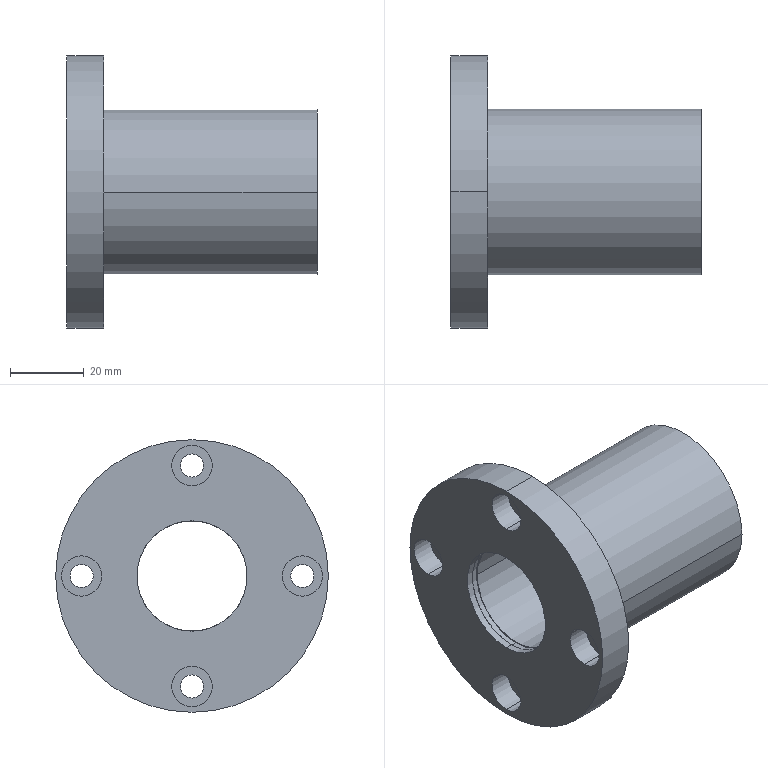Part | SolidWorks | features BaseBody 1 | 1 solid | 41 faces | box 68 x 74 x 74 mm | volume 84248 mm3 | cylinder 30 | plane 11 | commonest cylinder face diameters 6.3 x8 11 x8 30 x6 30.5 x4 45 x2 74 x2
STEP:
#1=CARTESIAN_POINT('',(0.,0.,37.));
#2=VERTEX_POINT('',#1);
#3=CARTESIAN_POINT('',(0.,0.,-37.));
#4=VERTEX_POINT('',#3);
#5=CARTESIAN_POINT('',(0.,0.,0.));
#6=DIRECTION('',(-1.,0.,0.));
#7=DIRECTION('',(0.,0.,-1.));
#8=AXIS2_PLACEMENT_3D('',#5,#6,#7);
#9=CIRCLE('',#8,37.);
#10=EDGE_CURVE('',#2,#4,#9,.T.);
#11=ORIENTED_EDGE('',*,*,#10,.F.);
#12=CARTESIAN_POINT('',(10.,0.,37.));
#13=VERTEX_POINT('',#12);
#14=CARTESIAN_POINT('',(0.,0.,37.));
#15=DIRECTION('',(1.,0.,0.));
#16=VECTOR('',#15,1000.);
#17=LINE('',#14,#16);
#18=EDGE_CURVE('',#2,#13,#17,.T.);
#19=ORIENTED_EDGE('',*,*,#18,.T.);
#20=CARTESIAN_POINT('',(10.,0.,-37.));
#21=VERTEX_POINT('',#20);
#22=CARTESIAN_POINT('',(10.,0.,0.));
#23=DIRECTION('',(1.,0.,0.));
#24=DIRECTION('',(0.,0.,-1.));
#25=AXIS2_PLACEMENT_3D('',#22,#23,#24);
#26=CIRCLE('',#25,37.);
#27=EDGE_CURVE('',#21,#13,#26,.T.);
#28=ORIENTED_EDGE('',*,*,#27,.F.);
#29=CARTESIAN_POINT('',(0.,0.,-37.));
#30=DIRECTION('',(1.,0.,0.));
#31=VECTOR('',#30,1000.);
#32=LINE('',#29,#31);
#33=EDGE_CURVE('',#4,#21,#32,.T.);
#34=ORIENTED_EDGE('',*,*,#33,.F.);
#35=EDGE_LOOP('',(#11,#19,#28,#34));
#36=FACE_OUTER_BOUND('',#35,.T.);
#37=CARTESIAN_POINT('',(0.,0.,0.));
#38=DIRECTION('',(1.,0.,0.));
#39=DIRECTION('',(0.,0.,-1.));
#40=AXIS2_PLACEMENT_3D('',#37,#38,#39);
#41=CYLINDRICAL_SURFACE('',#40,37.);
#42=ADVANCED_FACE('',(#36),#41,.T.);
#43=CARTESIAN_POINT('',(0.,0.,15.));
#44=VERTEX_POINT('',#43);
#45=CARTESIAN_POINT('',(0.,0.,-15.));
#46=VERTEX_POINT('',#45);
#47=CARTESIAN_POINT('',(0.,0.,0.));
#48=DIRECTION('',(1.,0.,0.));
#49=DIRECTION('',(0.,0.,-1.));
#50=AXIS2_PLACEMENT_3D('',#47,#48,#49);
#51=CIRCLE('',#50,15.);
#52=EDGE_CURVE('',#44,#46,#51,.T.);
#53=ORIENTED_EDGE('',*,*,#52,.F.);
#54=CARTESIAN_POINT('',(2.,0.,15.));
#55=VERTEX_POINT('',#54);
#56=CARTESIAN_POINT('',(0.,0.,15.));
#57=DIRECTION('',(1.,0.,0.));
#58=VECTOR('',#57,1000.);
#59=LINE('',#56,#58);
#60=EDGE_CURVE('',#44,#55,#59,.T.);
#61=ORIENTED_EDGE('',*,*,#60,.T.);
#62=CARTESIAN_POINT('',(2.,0.,-15.));
#63=VERTEX_POINT('',#62);
#64=CARTESIAN_POINT('',(2.,0.,0.));
#65=DIRECTION('',(1.,0.,0.));
#66=DIRECTION('',(0.,0.,-1.));
#67=AXIS2_PLACEMENT_3D('',#64,#65,#66);
#68=CIRCLE('',#67,15.);
#69=EDGE_CURVE('',#55,#63,#68,.T.);
#70=ORIENTED_EDGE('',*,*,#69,.T.);
#71=CARTESIAN_POINT('',(0.,0.,-15.));
#72=DIRECTION('',(1.,0.,0.));
#73=VECTOR('',#72,1000.);
#74=LINE('',#71,#73);
#75=EDGE_CURVE('',#46,#63,#74,.T.);
#76=ORIENTED_EDGE('',*,*,#75,.F.);
#77=EDGE_LOOP('',(#53,#61,#70,#76));
#78=FACE_OUTER_BOUND('',#77,.T.);
#79=CARTESIAN_POINT('',(0.,0.,0.));
#80=DIRECTION('',(1.,0.,0.));
#81=DIRECTION('',(0.,0.,-1.));
#82=AXIS2_PLACEMENT_3D('',#79,#80,#81);
#83=CYLINDRICAL_SURFACE('',#82,15.);
#84=ADVANCED_FACE('',(#78),#83,.F.);
#85=CARTESIAN_POINT('',(0.,30.,5.5));
#86=VERTEX_POINT('',#85);
#87=CARTESIAN_POINT('',(0.,30.,-5.5));
#88=VERTEX_POINT('',#87);
#89=CARTESIAN_POINT('',(0.,30.,0.));
#90=DIRECTION('',(1.,0.,0.));
#91=DIRECTION('',(0.,0.,-1.));
#92=AXIS2_PLACEMENT_3D('',#89,#90,#91);
#93=CIRCLE('',#92,5.5);
#94=EDGE_CURVE('',#86,#88,#93,.T.);
#95=ORIENTED_EDGE('',*,*,#94,.F.);
#96=CARTESIAN_POINT('',(6.3,30.,5.5));
#97=VERTEX_POINT('',#96);
#98=CARTESIAN_POINT('',(0.,30.,5.5));
#99=DIRECTION('',(1.,0.,0.));
#100=VECTOR('',#99,1000.);
#101=LINE('',#98,#100);
#102=EDGE_CURVE('',#86,#97,#101,.T.);
#103=ORIENTED_EDGE('',*,*,#102,.T.);
#104=CARTESIAN_POINT('',(6.3,30.,-5.5));
#105=VERTEX_POINT('',#104);
#106=CARTESIAN_POINT('',(6.3,30.,0.));
#107=DIRECTION('',(1.,0.,0.));
#108=DIRECTION('',(0.,0.,-1.));
#109=AXIS2_PLACEMENT_3D('',#106,#107,#108);
#110=CIRCLE('',#109,5.5);
#111=EDGE_CURVE('',#97,#105,#110,.T.);
#112=ORIENTED_EDGE('',*,*,#111,.T.);
#113=CARTESIAN_POINT('',(0.,30.,-5.5));
#114=DIRECTION('',(1.,0.,0.));
#115=VECTOR('',#114,1000.);
#116=LINE('',#113,#115);
#117=EDGE_CURVE('',#88,#105,#116,.T.);
#118=ORIENTED_EDGE('',*,*,#117,.F.);
#119=EDGE_LOOP('',(#95,#103,#112,#118));
#120=FACE_OUTER_BOUND('',#119,.T.);
#121=CARTESIAN_POINT('',(0.,30.,0.));
#122=DIRECTION('',(1.,0.,0.));
#123=DIRECTION('',(0.,0.,-1.));
#124=AXIS2_PLACEMENT_3D('',#121,#122,#123);
#125=CYLINDRICAL_SURFACE('',#124,5.5);
#126=ADVANCED_FACE('',(#120),#125,.F.);
#127=CARTESIAN_POINT('',(0.,0.,35.5));
#128=VERTEX_POINT('',#127);
#129=CARTESIAN_POINT('',(0.,0.,24.5));
#130=VERTEX_POINT('',#129);
#131=CARTESIAN_POINT('',(0.,0.,30.));
#132=DIRECTION('',(1.,0.,0.));
#133=DIRECTION('',(0.,0.,-1.));
#134=AXIS2_PLACEMENT_3D('',#131,#132,#133);
#135=CIRCLE('',#134,5.5);
#136=EDGE_CURVE('',#128,#130,#135,.T.);
#137=ORIENTED_EDGE('',*,*,#136,.F.);
#138=CARTESIAN_POINT('',(6.3,0.,35.5));
#139=VERTEX_POINT('',#138);
#140=CARTESIAN_POINT('',(0.,0.,35.5));
#141=DIRECTION('',(1.,0.,0.));
#142=VECTOR('',#141,1000.);
#143=LINE('',#140,#142);
#144=EDGE_CURVE('',#128,#139,#143,.T.);
#145=ORIENTED_EDGE('',*,*,#144,.T.);
#146=CARTESIAN_POINT('',(6.3,0.,24.5));
#147=VERTEX_POINT('',#146);
#148=CARTESIAN_POINT('',(6.3,0.,30.));
#149=DIRECTION('',(1.,0.,0.));
#150=DIRECTION('',(0.,0.,-1.));
#151=AXIS2_PLACEMENT_3D('',#148,#149,#150);
#152=CIRCLE('',#151,5.5);
#153=EDGE_CURVE('',#139,#147,#152,.T.);
#154=ORIENTED_EDGE('',*,*,#153,.T.);
#155=CARTESIAN_POINT('',(0.,0.,24.5));
#156=DIRECTION('',(1.,0.,0.));
#157=VECTOR('',#156,1000.);
#158=LINE('',#155,#157);
#159=EDGE_CURVE('',#130,#147,#158,.T.);
#160=ORIENTED_EDGE('',*,*,#159,.F.);
#161=EDGE_LOOP('',(#137,#145,#154,#160));
#162=FACE_OUTER_BOUND('',#161,.T.);
#163=CARTESIAN_POINT('',(0.,0.,30.));
#164=DIRECTION('',(1.,0.,0.));
#165=DIRECTION('',(0.,0.,-1.));
#166=AXIS2_PLACEMENT_3D('',#163,#164,#165);
#167=CYLINDRICAL_SURFACE('',#166,5.5);
#168=ADVANCED_FACE('',(#162),#167,.F.);
#169=CARTESIAN_POINT('',(0.,-30.,5.5));
#170=VERTEX_POINT('',#169);
#171=CARTESIAN_POINT('',(0.,-30.,-5.5));
#172=VERTEX_POINT('',#171);
#173=CARTESIAN_POINT('',(0.,-30.,0.));
#174=DIRECTION('',(1.,0.,0.));
#175=DIRECTION('',(0.,0.,-1.));
#176=AXIS2_PLACEMENT_3D('',#173,#174,#175);
#177=CIRCLE('',#176,5.5);
#178=EDGE_CURVE('',#170,#172,#177,.T.);
#179=ORIENTED_EDGE('',*,*,#178,.F.);
#180=CARTESIAN_POINT('',(6.3,-30.,5.5));
#181=VERTEX_POINT('',#180);
#182=CARTESIAN_POINT('',(0.,-30.,5.5));
#183=DIRECTION('',(1.,0.,0.));
#184=VECTOR('',#183,1000.);
#185=LINE('',#182,#184);
#186=EDGE_CURVE('',#170,#181,#185,.T.);
#187=ORIENTED_EDGE('',*,*,#186,.T.);
#188=CARTESIAN_POINT('',(6.3,-30.,-5.5));
#189=VERTEX_POINT('',#188);
#190=CARTESIAN_POINT('',(6.3,-30.,0.));
#191=DIRECTION('',(1.,0.,0.));
#192=DIRECTION('',(0.,0.,-1.));
#193=AXIS2_PLACEMENT_3D('',#190,#191,#192);
#194=CIRCLE('',#193,5.5);
#195=EDGE_CURVE('',#181,#189,#194,.T.);
#196=ORIENTED_EDGE('',*,*,#195,.T.);
#197=CARTESIAN_POINT('',(0.,-30.,-5.5));
#198=DIRECTION('',(1.,0.,0.));
#199=VECTOR('',#198,1000.);
#200=LINE('',#197,#199);
#201=EDGE_CURVE('',#172,#189,#200,.T.);
#202=ORIENTED_EDGE('',*,*,#201,.F.);
#203=EDGE_LOOP('',(#179,#187,#196,#202));
#204=FACE_OUTER_BOUND('',#203,.T.);
#205=CARTESIAN_POINT('',(0.,-30.,0.));
#206=DIRECTION('',(1.,0.,0.));
#207=DIRECTION('',(0.,0.,-1.));
#208=AXIS2_PLACEMENT_3D('',#205,#206,#207);
#209=CYLINDRICAL_SURFACE('',#208,5.5);
#210=ADVANCED_FACE('',(#204),#209,.F.);
#211=CARTESIAN_POINT('',(0.,0.,-24.5));
#212=VERTEX_POINT('',#211);
#213=CARTESIAN_POINT('',(0.,0.,-35.5));
#214=VERTEX_POINT('',#213);
#215=CARTESIAN_POINT('',(0.,0.,-30.));
#216=DIRECTION('',(1.,0.,0.));
#217=DIRECTION('',(0.,0.,-1.));
#218=AXIS2_PLACEMENT_3D('',#215,#216,#217);
#219=CIRCLE('',#218,5.5);
#220=EDGE_CURVE('',#212,#214,#219,.T.);
#221=ORIENTED_EDGE('',*,*,#220,.F.);
#222=CARTESIAN_POINT('',(6.3,0.,-24.5));
#223=VERTEX_POINT('',#222);
#224=CARTESIAN_POINT('',(0.,0.,-24.5));
#225=DIRECTION('',(1.,0.,0.));
#226=VECTOR('',#225,1000.);
#227=LINE('',#224,#226);
#228=EDGE_CURVE('',#212,#223,#227,.T.);
#229=ORIENTED_EDGE('',*,*,#228,.T.);
#230=CARTESIAN_POINT('',(6.3,0.,-35.5));
#231=VERTEX_POINT('',#230);
#232=CARTESIAN_POINT('',(6.3,0.,-30.));
#233=DIRECTION('',(1.,0.,0.));
#234=DIRECTION('',(0.,0.,-1.));
#235=AXIS2_PLACEMENT_3D('',#232,#233,#234);
#236=CIRCLE('',#235,5.5);
#237=EDGE_CURVE('',#223,#231,#236,.T.);
#238=ORIENTED_EDGE('',*,*,#237,.T.);
#239=CARTESIAN_POINT('',(0.,0.,-35.5));
#240=DIRECTION('',(1.,0.,0.));
#241=VECTOR('',#240,1000.);
#242=LINE('',#239,#241);
#243=EDGE_CURVE('',#214,#231,#242,.T.);
#244=ORIENTED_EDGE('',*,*,#243,.F.);
#245=EDGE_LOOP('',(#221,#229,#238,#244));
#246=FACE_OUTER_BOUND('',#245,.T.);
#247=CARTESIAN_POINT('',(0.,0.,-30.));
#248=DIRECTION('',(1.,0.,0.));
#249=DIRECTION('',(0.,0.,-1.));
#250=AXIS2_PLACEMENT_3D('',#247,#248,#249);
#251=CYLINDRICAL_SURFACE('',#250,5.5);
#252=ADVANCED_FACE('',(#246),#251,.F.);
#253=CARTESIAN_POINT('',(6.3,30.,-3.15));
#254=VERTEX_POINT('',#253);
#255=CARTESIAN_POINT('',(6.3,30.,3.15));
#256=VERTEX_POINT('',#255);
#257=CARTESIAN_POINT('',(6.3,30.,0.));
#258=DIRECTION('',(-1.,0.,0.));
#259=DIRECTION('',(0.,0.,-1.));
#260=AXIS2_PLACEMENT_3D('',#257,#258,#259);
#261=CIRCLE('',#260,3.15);
#262=EDGE_CURVE('',#254,#256,#261,.T.);
#263=ORIENTED_EDGE('',*,*,#262,.T.);
#264=CARTESIAN_POINT('',(10.,30.,3.15));
#265=VERTEX_POINT('',#264);
#266=CARTESIAN_POINT('',(6.3,30.,3.15));
#267=DIRECTION('',(1.,0.,0.));
#268=VECTOR('',#267,1000.);
#269=LINE('',#266,#268);
#270=EDGE_CURVE('',#256,#265,#269,.T.);
#271=ORIENTED_EDGE('',*,*,#270,.T.);
#272=CARTESIAN_POINT('',(10.,30.,-3.15));
#273=VERTEX_POINT('',#272);
#274=CARTESIAN_POINT('',(10.,30.,0.));
#275=DIRECTION('',(-1.,0.,0.));
#276=DIRECTION('',(0.,0.,-1.));
#277=AXIS2_PLACEMENT_3D('',#274,#275,#276);
#278=CIRCLE('',#277,3.15);
#279=EDGE_CURVE('',#273,#265,#278,.T.);
#280=ORIENTED_EDGE('',*,*,#279,.F.);
#281=CARTESIAN_POINT('',(6.3,30.,-3.15));
#282=DIRECTION('',(1.,0.,0.));
#283=VECTOR('',#282,1000.);
#284=LINE('',#281,#283);
#285=EDGE_CURVE('',#254,#273,#284,.T.);
#286=ORIENTED_EDGE('',*,*,#285,.F.);
#287=EDGE_LOOP('',(#263,#271,#280,#286));
#288=FACE_OUTER_BOUND('',#287,.T.);
#289=CARTESIAN_POINT('',(6.3,30.,0.));
#290=DIRECTION('',(1.,0.,0.));
#291=DIRECTION('',(0.,0.,-1.));
#292=AXIS2_PLACEMENT_3D('',#289,#290,#291);
#293=CYLINDRICAL_SURFACE('',#292,3.15);
#294=ADVANCED_FACE('',(#288),#293,.F.);
#295=CARTESIAN_POINT('',(6.3,0.,26.85));
#296=VERTEX_POINT('',#295);
#297=CARTESIAN_POINT('',(6.3,0.,33.15));
#298=VERTEX_POINT('',#297);
#299=CARTESIAN_POINT('',(6.3,0.,30.));
#300=DIRECTION('',(-1.,0.,0.));
#301=DIRECTION('',(0.,0.,-1.));
#302=AXIS2_PLACEMENT_3D('',#299,#300,#301);
#303=CIRCLE('',#302,3.15);
#304=EDGE_CURVE('',#296,#298,#303,.T.);
#305=ORIENTED_EDGE('',*,*,#304,.T.);
#306=CARTESIAN_POINT('',(10.,0.,33.15));
#307=VERTEX_POINT('',#306);
#308=CARTESIAN_POINT('',(6.3,0.,33.15));
#309=DIRECTION('',(1.,0.,0.));
#310=VECTOR('',#309,1000.);
#311=LINE('',#308,#310);
#312=EDGE_CURVE('',#298,#307,#311,.T.);
#313=ORIENTED_EDGE('',*,*,#312,.T.);
#314=CARTESIAN_POINT('',(10.,0.,26.85));
#315=VERTEX_POINT('',#314);
#316=CARTESIAN_POINT('',(10.,0.,30.));
#317=DIRECTION('',(-1.,0.,0.));
#318=DIRECTION('',(0.,0.,-1.));
#319=AXIS2_PLACEMENT_3D('',#316,#317,#318);
#320=CIRCLE('',#319,3.15);
#321=EDGE_CURVE('',#315,#307,#320,.T.);
#322=ORIENTED_EDGE('',*,*,#321,.F.);
#323=CARTESIAN_POINT('',(6.3,0.,26.85));
#324=DIRECTION('',(1.,0.,0.));
#325=VECTOR('',#324,1000.);
#326=LINE('',#323,#325);
#327=EDGE_CURVE('',#296,#315,#326,.T.);
#328=ORIENTED_EDGE('',*,*,#327,.F.);
#329=EDGE_LOOP('',(#305,#313,#322,#328));
#330=FACE_OUTER_BOUND('',#329,.T.);
#331=CARTESIAN_POINT('',(6.3,0.,30.));
#332=DIRECTION('',(1.,0.,0.));
#333=DIRECTION('',(0.,0.,-1.));
#334=AXIS2_PLACEMENT_3D('',#331,#332,#333);
#335=CYLINDRICAL_SURFACE('',#334,3.15);
#336=ADVANCED_FACE('',(#330),#335,.F.);
#337=CARTESIAN_POINT('',(6.3,-30.,-3.15));
#338=VERTEX_POINT('',#337);
#339=CARTESIAN_POINT('',(6.3,-30.,3.15));
#340=VERTEX_POINT('',#339);
#341=CARTESIAN_POINT('',(6.3,-30.,0.));
#342=DIRECTION('',(-1.,0.,0.));
#343=DIRECTION('',(0.,0.,-1.));
#344=AXIS2_PLACEMENT_3D('',#341,#342,#343);
#345=CIRCLE('',#344,3.15);
#346=EDGE_CURVE('',#338,#340,#345,.T.);
#347=ORIENTED_EDGE('',*,*,#346,.T.);
#348=CARTESIAN_POINT('',(10.,-30.,3.15));
#349=VERTEX_POINT('',#348);
#350=CARTESIAN_POINT('',(6.3,-30.,3.15));
#351=DIRECTION('',(1.,0.,0.));
#352=VECTOR('',#351,1000.);
#353=LINE('',#350,#352);
#354=EDGE_CURVE('',#340,#349,#353,.T.);
#355=ORIENTED_EDGE('',*,*,#354,.T.);
#356=CARTESIAN_POINT('',(10.,-30.,-3.15));
#357=VERTEX_POINT('',#356);
#358=CARTESIAN_POINT('',(10.,-30.,0.));
#359=DIRECTION('',(-1.,0.,0.));
#360=DIRECTION('',(0.,0.,-1.));
#361=AXIS2_PLACEMENT_3D('',#358,#359,#360);
#362=CIRCLE('',#361,3.15);
#363=EDGE_CURVE('',#357,#349,#362,.T.);
#364=ORIENTED_EDGE('',*,*,#363,.F.);
#365=CARTESIAN_POINT('',(6.3,-30.,-3.15));
#366=DIRECTION('',(1.,0.,0.));
#367=VECTOR('',#366,1000.);
#368=LINE('',#365,#367);
#369=EDGE_CURVE('',#338,#357,#368,.T.);
#370=ORIENTED_EDGE('',*,*,#369,.F.);
#371=EDGE_LOOP('',(#347,#355,#364,#370));
#372=FACE_OUTER_BOUND('',#371,.T.);
#373=CARTESIAN_POINT('',(6.3,-30.,0.));
#374=DIRECTION('',(1.,0.,0.));
#375=DIRECTION('',(0.,0.,-1.));
#376=AXIS2_PLACEMENT_3D('',#373,#374,#375);
#377=CYLINDRICAL_SURFACE('',#376,3.15);
#378=ADVANCED_FACE('',(#372),#377,.F.);
#379=CARTESIAN_POINT('',(6.3,0.,-33.15));
#380=VERTEX_POINT('',#379);
#381=CARTESIAN_POINT('',(6.3,0.,-26.85));
#382=VERTEX_POINT('',#381);
#383=CARTESIAN_POINT('',(6.3,0.,-30.));
#384=DIRECTION('',(-1.,0.,0.));
#385=DIRECTION('',(0.,0.,-1.));
#386=AXIS2_PLACEMENT_3D('',#383,#384,#385);
#387=CIRCLE('',#386,3.15);
#388=EDGE_CURVE('',#380,#382,#387,.T.);
#389=ORIENTED_EDGE('',*,*,#388,.T.);
#390=CARTESIAN_POINT('',(10.,0.,-26.85));
#391=VERTEX_POINT('',#390);
#392=CARTESIAN_POINT('',(6.3,0.,-26.85));
#393=DIRECTION('',(1.,0.,0.));
#394=VECTOR('',#393,1000.);
#395=LINE('',#392,#394);
#396=EDGE_CURVE('',#382,#391,#395,.T.);
#397=ORIENTED_EDGE('',*,*,#396,.T.);
#398=CARTESIAN_POINT('',(10.,0.,-33.15));
#399=VERTEX_POINT('',#398);
#400=CARTESIAN_POINT('',(10.,0.,-30.));
#401=DIRECTION('',(-1.,0.,0.));
#402=DIRECTION('',(0.,0.,-1.));
#403=AXIS2_PLACEMENT_3D('',#400,#401,#402);
#404=CIRCLE('',#403,3.15);
#405=EDGE_CURVE('',#399,#391,#404,.T.);
#406=ORIENTED_EDGE('',*,*,#405,.F.);
#407=CARTESIAN_POINT('',(6.3,0.,-33.15));
#408=DIRECTION('',(1.,0.,0.));
#409=VECTOR('',#408,1000.);
#410=LINE('',#407,#409);
#411=EDGE_CURVE('',#380,#399,#410,.T.);
#412=ORIENTED_EDGE('',*,*,#411,.F.);
#413=EDGE_LOOP('',(#389,#397,#406,#412));
#414=FACE_OUTER_BOUND('',#413,.T.);
#415=CARTESIAN_POINT('',(6.3,0.,-30.));
#416=DIRECTION('',(1.,0.,0.));
#417=DIRECTION('',(0.,0.,-1.));
#418=AXIS2_PLACEMENT_3D('',#415,#416,#417);
#419=CYLINDRICAL_SURFACE('',#418,3.15);
#420=ADVANCED_FACE('',(#414),#419,.F.);
#421=CARTESIAN_POINT('',(10.,-22.5,0.));
#422=VERTEX_POINT('',#421);
#423=CARTESIAN_POINT('',(10.,22.5,0.));
#424=VERTEX_POINT('',#423);
#425=CARTESIAN_POINT('',(10.,0.,0.));
#426=DIRECTION('',(-1.,0.,0.));
#427=DIRECTION('',(0.,1.,0.));
#428=AXIS2_PLACEMENT_3D('',#425,#426,#427);
#429=CIRCLE('',#428,22.5);
#430=EDGE_CURVE('',#422,#424,#429,.T.);
#431=ORIENTED_EDGE('',*,*,#430,.F.);
#432=CARTESIAN_POINT('',(68.,-22.5,0.));
#433=VERTEX_POINT('',#432);
#434=CARTESIAN_POINT('',(10.,-22.5,0.));
#435=DIRECTION('',(1.,0.,0.));
#436=VECTOR('',#435,1000.);
#437=LINE('',#434,#436);
#438=EDGE_CURVE('',#422,#433,#437,.T.);
#439=ORIENTED_EDGE('',*,*,#438,.T.);
#440=CARTESIAN_POINT('',(68.,22.5,0.));
#441=VERTEX_POINT('',#440);
#442=CARTESIAN_POINT('',(68.,0.,0.));
#443=DIRECTION('',(1.,0.,0.));
#444=DIRECTION('',(0.,1.,0.));
#445=AXIS2_PLACEMENT_3D('',#442,#443,#444);
#446=CIRCLE('',#445,22.5);
#447=EDGE_CURVE('',#441,#433,#446,.T.);
#448=ORIENTED_EDGE('',*,*,#447,.F.);
#449=CARTESIAN_POINT('',(10.,22.5,0.));
#450=DIRECTION('',(1.,0.,0.));
#451=VECTOR('',#450,1000.);
#452=LINE('',#449,#451);
#453=EDGE_CURVE('',#424,#441,#452,.T.);
#454=ORIENTED_EDGE('',*,*,#453,.F.);
#455=EDGE_LOOP('',(#431,#439,#448,#454));
#456=FACE_OUTER_BOUND('',#455,.T.);
#457=CARTESIAN_POINT('',(10.,0.,0.));
#458=DIRECTION('',(1.,0.,0.));
#459=DIRECTION('',(0.,1.,0.));
#460=AXIS2_PLACEMENT_3D('',#457,#458,#459);
#461=CYLINDRICAL_SURFACE('',#460,22.5);
#462=ADVANCED_FACE('',(#456),#461,.T.);
#463=CARTESIAN_POINT('',(2.,0.,15.25));
#464=VERTEX_POINT('',#463);
#465=CARTESIAN_POINT('',(2.,0.,-15.25));
#466=VERTEX_POINT('',#465);
#467=CARTESIAN_POINT('',(2.,0.,0.));
#468=DIRECTION('',(1.,0.,0.));
#469=DIRECTION('',(0.,0.,-1.));
#470=AXIS2_PLACEMENT_3D('',#467,#468,#469);
#471=CIRCLE('',#470,15.25);
#472=EDGE_CURVE('',#464,#466,#471,.T.);
#473=ORIENTED_EDGE('',*,*,#472,.F.);
#474=CARTESIAN_POINT('',(3.75,0.,15.25));
#475=VERTEX_POINT('',#474);
#476=CARTESIAN_POINT('',(2.,0.,15.25));
#477=DIRECTION('',(1.,0.,0.));
#478=VECTOR('',#477,1000.);
#479=LINE('',#476,#478);
#480=EDGE_CURVE('',#464,#475,#479,.T.);
#481=ORIENTED_EDGE('',*,*,#480,.T.);
#482=CARTESIAN_POINT('',(3.75,0.,-15.25));
#483=VERTEX_POINT('',#482);
#484=CARTESIAN_POINT('',(3.75,0.,0.));
#485=DIRECTION('',(1.,0.,0.));
#486=DIRECTION('',(0.,0.,-1.));
#487=AXIS2_PLACEMENT_3D('',#484,#485,#486);
#488=CIRCLE('',#487,15.25);
#489=EDGE_CURVE('',#475,#483,#488,.T.);
#490=ORIENTED_EDGE('',*,*,#489,.T.);
#491=CARTESIAN_POINT('',(2.,0.,-15.25));
#492=DIRECTION('',(1.,0.,0.));
#493=VECTOR('',#492,1000.);
#494=LINE('',#491,#493);
#495=EDGE_CURVE('',#466,#483,#494,.T.);
#496=ORIENTED_EDGE('',*,*,#495,.F.);
#497=EDGE_LOOP('',(#473,#481,#490,#496));
#498=FACE_OUTER_BOUND('',#497,.T.);
#499=CARTESIAN_POINT('',(2.,0.,0.));
#500=DIRECTION('',(1.,0.,0.));
#501=DIRECTION('',(0.,0.,-1.));
#502=AXIS2_PLACEMENT_3D('',#499,#500,#501);
#503=CYLINDRICAL_SURFACE('',#502,15.25);
#504=ADVANCED_FACE('',(#498),#503,.F.);
#505=CARTESIAN_POINT('',(66.,0.,-15.));
#506=VERTEX_POINT('',#505);
#507=CARTESIAN_POINT('',(66.,0.,15.));
#508=VERTEX_POINT('',#507);
#509=CARTESIAN_POINT('',(66.,0.,0.));
#510=DIRECTION('',(-1.,0.,0.));
#511=DIRECTION('',(0.,0.,-1.));
#512=AXIS2_PLACEMENT_3D('',#509,#510,#511);
#513=CIRCLE('',#512,15.);
#514=EDGE_CURVE('',#506,#508,#513,.T.);
#515=ORIENTED_EDGE('',*,*,#514,.T.);
#516=CARTESIAN_POINT('',(68.,0.,15.));
#517=VERTEX_POINT('',#516);
#518=CARTESIAN_POINT('',(66.,0.,15.));
#519=DIRECTION('',(1.,0.,0.));
#520=VECTOR('',#519,1000.);
#521=LINE('',#518,#520);
#522=EDGE_CURVE('',#508,#517,#521,.T.);
#523=ORIENTED_EDGE('',*,*,#522,.T.);
#524=CARTESIAN_POINT('',(68.,0.,-15.));
#525=VERTEX_POINT('',#524);
#526=CARTESIAN_POINT('',(68.,0.,0.));
#527=DIRECTION('',(-1.,0.,0.));
#528=DIRECTION('',(0.,0.,-1.));
#529=AXIS2_PLACEMENT_3D('',#526,#527,#528);
#530=CIRCLE('',#529,15.);
#531=EDGE_CURVE('',#525,#517,#530,.T.);
#532=ORIENTED_EDGE('',*,*,#531,.F.);
#533=CARTESIAN_POINT('',(66.,0.,-15.));
#534=DIRECTION('',(1.,0.,0.));
#535=VECTOR('',#534,1000.);
#536=LINE('',#533,#535);
#537=EDGE_CURVE('',#506,#525,#536,.T.);
#538=ORIENTED_EDGE('',*,*,#537,.F.);
#539=EDGE_LOOP('',(#515,#523,#532,#538));
#540=FACE_OUTER_BOUND('',#539,.T.);
#541=CARTESIAN_POINT('',(66.,0.,0.));
#542=DIRECTION('',(1.,0.,0.));
#543=DIRECTION('',(0.,0.,-1.));
#544=AXIS2_PLACEMENT_3D('',#541,#542,#543);
#545=CYLINDRICAL_SURFACE('',#544,15.);
#546=ADVANCED_FACE('',(#540),#545,.F.);
#547=CARTESIAN_POINT('',(3.75,-15.,0.));
#548=VERTEX_POINT('',#547);
#549=CARTESIAN_POINT('',(3.75,15.,0.));
#550=VERTEX_POINT('',#549);
#551=CARTESIAN_POINT('',(3.75,0.,0.));
#552=DIRECTION('',(1.,0.,0.));
#553=DIRECTION('',(0.,1.,0.));
#554=AXIS2_PLACEMENT_3D('',#551,#552,#553);
#555=CIRCLE('',#554,15.);
#556=EDGE_CURVE('',#548,#550,#555,.T.);
#557=ORIENTED_EDGE('',*,*,#556,.F.);
#558=CARTESIAN_POINT('',(64.25,-15.,0.));
#559=VERTEX_POINT('',#558);
#560=CARTESIAN_POINT('',(3.75,-15.,0.));
#561=DIRECTION('',(1.,0.,0.));
#562=VECTOR('',#561,1000.);
#563=LINE('',#560,#562);
#564=EDGE_CURVE('',#548,#559,#563,.T.);
#565=ORIENTED_EDGE('',*,*,#564,.T.);
#566=CARTESIAN_POINT('',(64.25,15.,0.));
#567=VERTEX_POINT('',#566);
#568=CARTESIAN_POINT('',(64.25,0.,0.));
#569=DIRECTION('',(1.,0.,0.));
#570=DIRECTION('',(0.,1.,0.));
#571=AXIS2_PLACEMENT_3D('',#568,#569,#570);
#572=CIRCLE('',#571,15.);
#573=EDGE_CURVE('',#559,#567,#572,.T.);
#574=ORIENTED_EDGE('',*,*,#573,.T.);
#575=CARTESIAN_POINT('',(3.75,15.,0.));
#576=DIRECTION('',(1.,0.,0.));
#577=VECTOR('',#576,1000.);
#578=LINE('',#575,#577);
#579=EDGE_CURVE('',#550,#567,#578,.T.);
#580=ORIENTED_EDGE('',*,*,#579,.F.);
#581=EDGE_LOOP('',(#557,#565,#574,#580));
#582=FACE_OUTER_BOUND('',#581,.T.);
#583=CARTESIAN_POINT('',(3.75,0.,0.));
#584=DIRECTION('',(1.,0.,0.));
#585=DIRECTION('',(0.,1.,0.));
#586=AXIS2_PLACEMENT_3D('',#583,#584,#585);
#587=CYLINDRICAL_SURFACE('',#586,15.);
#588=ADVANCED_FACE('',(#582),#587,.F.);
#589=CARTESIAN_POINT('',(64.25,0.,-15.25));
#590=VERTEX_POINT('',#589);
#591=CARTESIAN_POINT('',(64.25,0.,15.25));
#592=VERTEX_POINT('',#591);
#593=CARTESIAN_POINT('',(64.25,0.,0.));
#594=DIRECTION('',(-1.,0.,0.));
#595=DIRECTION('',(0.,0.,-1.));
#596=AXIS2_PLACEMENT_3D('',#593,#594,#595);
#597=CIRCLE('',#596,15.25);
#598=EDGE_CURVE('',#590,#592,#597,.T.);
#599=ORIENTED_EDGE('',*,*,#598,.T.);
#600=CARTESIAN_POINT('',(66.,0.,15.25));
#601=VERTEX_POINT('',#600);
#602=CARTESIAN_POINT('',(64.25,0.,15.25));
#603=DIRECTION('',(1.,0.,0.));
#604=VECTOR('',#603,1000.);
#605=LINE('',#602,#604);
#606=EDGE_CURVE('',#592,#601,#605,.T.);
#607=ORIENTED_EDGE('',*,*,#606,.T.);
#608=CARTESIAN_POINT('',(66.,0.,-15.25));
#609=VERTEX_POINT('',#608);
#610=CARTESIAN_POINT('',(66.,0.,0.));
#611=DIRECTION('',(-1.,0.,0.));
#612=DIRECTION('',(0.,0.,-1.));
#613=AXIS2_PLACEMENT_3D('',#610,#611,#612);
#614=CIRCLE('',#613,15.25);
#615=EDGE_CURVE('',#609,#601,#614,.T.);
#616=ORIENTED_EDGE('',*,*,#615,.F.);
#617=CARTESIAN_POINT('',(64.25,0.,-15.25));
#618=DIRECTION('',(1.,0.,0.));
#619=VECTOR('',#618,1000.);
#620=LINE('',#617,#619);
#621=EDGE_CURVE('',#590,#609,#620,.T.);
#622=ORIENTED_EDGE('',*,*,#621,.F.);
#623=EDGE_LOOP('',(#599,#607,#616,#622));
#624=FACE_OUTER_BOUND('',#623,.T.);
#625=CARTESIAN_POINT('',(64.25,0.,0.));
#626=DIRECTION('',(1.,0.,0.));
#627=DIRECTION('',(0.,0.,-1.));
#628=AXIS2_PLACEMENT_3D('',#625,#626,#627);
#629=CYLINDRICAL_SURFACE('',#628,15.25);
#630=ADVANCED_FACE('',(#624),#629,.F.);
#631=ORIENTED_EDGE('',*,*,#18,.F.);
#632=CARTESIAN_POINT('',(0.,0.,0.));
#633=DIRECTION('',(-1.,0.,0.));
#634=DIRECTION('',(0.,0.,-1.));
#635=AXIS2_PLACEMENT_3D('',#632,#633,#634);
#636=CIRCLE('',#635,37.);
#637=EDGE_CURVE('',#4,#2,#636,.T.);
#638=ORIENTED_EDGE('',*,*,#637,.F.);
#639=ORIENTED_EDGE('',*,*,#33,.T.);
#640=CARTESIAN_POINT('',(10.,0.,0.));
#641=DIRECTION('',(1.,0.,0.));
#642=DIRECTION('',(0.,0.,-1.));
#643=AXIS2_PLACEMENT_3D('',#640,#641,#642);
#644=CIRCLE('',#643,37.);
#645=EDGE_CURVE('',#13,#21,#644,.T.);
#646=ORIENTED_EDGE('',*,*,#645,.F.);
#647=EDGE_LOOP('',(#631,#638,#639,#646));
#648=FACE_OUTER_BOUND('',#647,.T.);
#649=CARTESIAN_POINT('',(0.,0.,0.));
#650=DIRECTION('',(1.,0.,0.));
#651=DIRECTION('',(0.,0.,-1.));
#652=AXIS2_PLACEMENT_3D('',#649,#650,#651);
#653=CYLINDRICAL_SURFACE('',#652,37.);
#654=ADVANCED_FACE('',(#648),#653,.T.);
#655=CARTESIAN_POINT('',(0.,0.,0.));
#656=DIRECTION('',(1.,0.,0.));
#657=DIRECTION('',(0.,0.,-1.));
#658=AXIS2_PLACEMENT_3D('',#655,#656,#657);
#659=CIRCLE('',#658,15.);
#660=EDGE_CURVE('',#46,#44,#659,.T.);
#661=ORIENTED_EDGE('',*,*,#660,.T.);
#662=ORIENTED_EDGE('',*,*,#52,.T.);
#663=EDGE_LOOP('',(#661,#662));
#664=FACE_BOUND('',#663,.T.);
#665=CARTESIAN_POINT('',(0.,30.,0.));
#666=DIRECTION('',(1.,0.,0.));
#667=DIRECTION('',(0.,0.,-1.));
#668=AXIS2_PLACEMENT_3D('',#665,#666,#667);
#669=CIRCLE('',#668,5.5);
#670=EDGE_CURVE('',#88,#86,#669,.T.);
#671=ORIENTED_EDGE('',*,*,#670,.T.);
#672=ORIENTED_EDGE('',*,*,#94,.T.);
#673=EDGE_LOOP('',(#671,#672));
#674=FACE_BOUND('',#673,.T.);
#675=CARTESIAN_POINT('',(0.,0.,30.));
#676=DIRECTION('',(1.,0.,0.));
#677=DIRECTION('',(0.,0.,-1.));
#678=AXIS2_PLACEMENT_3D('',#675,#676,#677);
#679=CIRCLE('',#678,5.5);
#680=EDGE_CURVE('',#130,#128,#679,.T.);
#681=ORIENTED_EDGE('',*,*,#680,.T.);
#682=ORIENTED_EDGE('',*,*,#136,.T.);
#683=EDGE_LOOP('',(#681,#682));
#684=FACE_BOUND('',#683,.T.);
#685=CARTESIAN_POINT('',(0.,-30.,0.));
#686=DIRECTION('',(1.,0.,0.));
#687=DIRECTION('',(0.,0.,-1.));
#688=AXIS2_PLACEMENT_3D('',#685,#686,#687);
#689=CIRCLE('',#688,5.5);
#690=EDGE_CURVE('',#172,#170,#689,.T.);
#691=ORIENTED_EDGE('',*,*,#690,.T.);
#692=ORIENTED_EDGE('',*,*,#178,.T.);
#693=EDGE_LOOP('',(#691,#692));
#694=FACE_BOUND('',#693,.T.);
#695=CARTESIAN_POINT('',(0.,0.,-30.));
#696=DIRECTION('',(1.,0.,0.));
#697=DIRECTION('',(0.,0.,-1.));
#698=AXIS2_PLACEMENT_3D('',#695,#696,#697);
#699=CIRCLE('',#698,5.5);
#700=EDGE_CURVE('',#214,#212,#699,.T.);
#701=ORIENTED_EDGE('',*,*,#700,.T.);
#702=ORIENTED_EDGE('',*,*,#220,.T.);
#703=EDGE_LOOP('',(#701,#702));
#704=FACE_BOUND('',#703,.T.);
#705=ORIENTED_EDGE('',*,*,#637,.T.);
#706=ORIENTED_EDGE('',*,*,#10,.T.);
#707=EDGE_LOOP('',(#705,#706));
#708=FACE_OUTER_BOUND('',#707,.T.);
#709=CARTESIAN_POINT('',(0.,-37.444,-37.444));
#710=DIRECTION('',(-1.,0.,0.));
#711=DIRECTION('',(0.,0.,1.));
#712=AXIS2_PLACEMENT_3D('',#709,#710,#711);
#713=PLANE('',#712);
#714=ADVANCED_FACE('',(#664,#674,#684,#694,#704,#708),#713,.T.);
#715=ORIENTED_EDGE('',*,*,#279,.T.);
#716=CARTESIAN_POINT('',(10.,30.,0.));
#717=DIRECTION('',(-1.,0.,0.));
#718=DIRECTION('',(0.,0.,-1.));
#719=AXIS2_PLACEMENT_3D('',#716,#717,#718);
#720=CIRCLE('',#719,3.15);
#721=EDGE_CURVE('',#265,#273,#720,.T.);
#722=ORIENTED_EDGE('',*,*,#721,.T.);
#723=EDGE_LOOP('',(#715,#722));
#724=FACE_BOUND('',#723,.T.);
#725=ORIENTED_EDGE('',*,*,#321,.T.);
#726=CARTESIAN_POINT('',(10.,0.,30.));
#727=DIRECTION('',(-1.,0.,0.));
#728=DIRECTION('',(0.,0.,-1.));
#729=AXIS2_PLACEMENT_3D('',#726,#727,#728);
#730=CIRCLE('',#729,3.15);
#731=EDGE_CURVE('',#307,#315,#730,.T.);
#732=ORIENTED_EDGE('',*,*,#731,.T.);
#733=EDGE_LOOP('',(#725,#732));
#734=FACE_BOUND('',#733,.T.);
#735=ORIENTED_EDGE('',*,*,#363,.T.);
#736=CARTESIAN_POINT('',(10.,-30.,0.));
#737=DIRECTION('',(-1.,0.,0.));
#738=DIRECTION('',(0.,0.,-1.));
#739=AXIS2_PLACEMENT_3D('',#736,#737,#738);
#740=CIRCLE('',#739,3.15);
#741=EDGE_CURVE('',#349,#357,#740,.T.);
#742=ORIENTED_EDGE('',*,*,#741,.T.);
#743=EDGE_LOOP('',(#735,#742));
#744=FACE_BOUND('',#743,.T.);
#745=ORIENTED_EDGE('',*,*,#405,.T.);
#746=CARTESIAN_POINT('',(10.,0.,-30.));
#747=DIRECTION('',(-1.,0.,0.));
#748=DIRECTION('',(0.,0.,-1.));
#749=AXIS2_PLACEMENT_3D('',#746,#747,#748);
#750=CIRCLE('',#749,3.15);
#751=EDGE_CURVE('',#391,#399,#750,.T.);
#752=ORIENTED_EDGE('',*,*,#751,.T.);
#753=EDGE_LOOP('',(#745,#752));
#754=FACE_BOUND('',#753,.T.);
#755=CARTESIAN_POINT('',(10.,0.,0.));
#756=DIRECTION('',(-1.,0.,0.));
#757=DIRECTION('',(0.,1.,0.));
#758=AXIS2_PLACEMENT_3D('',#755,#756,#757);
#759=CIRCLE('',#758,22.5);
#760=EDGE_CURVE('',#424,#422,#759,.T.);
#761=ORIENTED_EDGE('',*,*,#760,.T.);
#762=ORIENTED_EDGE('',*,*,#430,.T.);
#763=EDGE_LOOP('',(#761,#762));
#764=FACE_BOUND('',#763,.T.);
#765=ORIENTED_EDGE('',*,*,#27,.T.);
#766=ORIENTED_EDGE('',*,*,#645,.T.);
#767=EDGE_LOOP('',(#765,#766));
#768=FACE_OUTER_BOUND('',#767,.T.);
#769=CARTESIAN_POINT('',(10.,-37.444,-37.444));
#770=DIRECTION('',(1.,0.,0.));
#771=DIRECTION('',(0.,1.,0.));
#772=AXIS2_PLACEMENT_3D('',#769,#770,#771);
#773=PLANE('',#772);
#774=ADVANCED_FACE('',(#724,#734,#744,#754,#764,#768),#773,.T.);
#775=ORIENTED_EDGE('',*,*,#60,.F.);
#776=ORIENTED_EDGE('',*,*,#660,.F.);
#777=ORIENTED_EDGE('',*,*,#75,.T.);
#778=CARTESIAN_POINT('',(2.,0.,0.));
#779=DIRECTION('',(1.,0.,0.));
#780=DIRECTION('',(0.,0.,-1.));
#781=AXIS2_PLACEMENT_3D('',#778,#779,#780);
#782=CIRCLE('',#781,15.);
#783=EDGE_CURVE('',#63,#55,#782,.T.);
#784=ORIENTED_EDGE('',*,*,#783,.T.);
#785=EDGE_LOOP('',(#775,#776,#777,#784));
#786=FACE_OUTER_BOUND('',#785,.T.);
#787=CARTESIAN_POINT('',(0.,0.,0.));
#788=DIRECTION('',(1.,0.,0.));
#789=DIRECTION('',(0.,0.,-1.));
#790=AXIS2_PLACEMENT_3D('',#787,#788,#789);
#791=CYLINDRICAL_SURFACE('',#790,15.);
#792=ADVANCED_FACE('',(#786),#791,.F.);
#793=ORIENTED_EDGE('',*,*,#102,.F.);
#794=ORIENTED_EDGE('',*,*,#670,.F.);
#795=ORIENTED_EDGE('',*,*,#117,.T.);
#796=CARTESIAN_POINT('',(6.3,30.,0.));
#797=DIRECTION('',(1.,0.,0.));
#798=DIRECTION('',(0.,0.,-1.));
#799=AXIS2_PLACEMENT_3D('',#796,#797,#798);
#800=CIRCLE('',#799,5.5);
#801=EDGE_CURVE('',#105,#97,#800,.T.);
#802=ORIENTED_EDGE('',*,*,#801,.T.);
#803=EDGE_LOOP('',(#793,#794,#795,#802));
#804=FACE_OUTER_BOUND('',#803,.T.);
#805=CARTESIAN_POINT('',(0.,30.,0.));
#806=DIRECTION('',(1.,0.,0.));
#807=DIRECTION('',(0.,0.,-1.));
#808=AXIS2_PLACEMENT_3D('',#805,#806,#807);
#809=CYLINDRICAL_SURFACE('',#808,5.5);
#810=ADVANCED_FACE('',(#804),#809,.F.);
#811=ORIENTED_EDGE('',*,*,#144,.F.);
#812=ORIENTED_EDGE('',*,*,#680,.F.);
#813=ORIENTED_EDGE('',*,*,#159,.T.);
#814=CARTESIAN_POINT('',(6.3,0.,30.));
#815=DIRECTION('',(1.,0.,0.));
#816=DIRECTION('',(0.,0.,-1.));
#817=AXIS2_PLACEMENT_3D('',#814,#815,#816);
#818=CIRCLE('',#817,5.5);
#819=EDGE_CURVE('',#147,#139,#818,.T.);
#820=ORIENTED_EDGE('',*,*,#819,.T.);
#821=EDGE_LOOP('',(#811,#812,#813,#820));
#822=FACE_OUTER_BOUND('',#821,.T.);
#823=CARTESIAN_POINT('',(0.,0.,30.));
#824=DIRECTION('',(1.,0.,0.));
#825=DIRECTION('',(0.,0.,-1.));
#826=AXIS2_PLACEMENT_3D('',#823,#824,#825);
#827=CYLINDRICAL_SURFACE('',#826,5.5);
#828=ADVANCED_FACE('',(#822),#827,.F.);
#829=ORIENTED_EDGE('',*,*,#186,.F.);
#830=ORIENTED_EDGE('',*,*,#690,.F.);
#831=ORIENTED_EDGE('',*,*,#201,.T.);
#832=CARTESIAN_POINT('',(6.3,-30.,0.));
#833=DIRECTION('',(1.,0.,0.));
#834=DIRECTION('',(0.,0.,-1.));
#835=AXIS2_PLACEMENT_3D('',#832,#833,#834);
#836=CIRCLE('',#835,5.5);
#837=EDGE_CURVE('',#189,#181,#836,.T.);
#838=ORIENTED_EDGE('',*,*,#837,.T.);
#839=EDGE_LOOP('',(#829,#830,#831,#838));
#840=FACE_OUTER_BOUND('',#839,.T.);
#841=CARTESIAN_POINT('',(0.,-30.,0.));
#842=DIRECTION('',(1.,0.,0.));
#843=DIRECTION('',(0.,0.,-1.));
#844=AXIS2_PLACEMENT_3D('',#841,#842,#843);
#845=CYLINDRICAL_SURFACE('',#844,5.5);
#846=ADVANCED_FACE('',(#840),#845,.F.);
#847=ORIENTED_EDGE('',*,*,#228,.F.);
#848=ORIENTED_EDGE('',*,*,#700,.F.);
#849=ORIENTED_EDGE('',*,*,#243,.T.);
#850=CARTESIAN_POINT('',(6.3,0.,-30.));
#851=DIRECTION('',(1.,0.,0.));
#852=DIRECTION('',(0.,0.,-1.));
#853=AXIS2_PLACEMENT_3D('',#850,#851,#852);
#854=CIRCLE('',#853,5.5);
#855=EDGE_CURVE('',#231,#223,#854,.T.);
#856=ORIENTED_EDGE('',*,*,#855,.T.);
#857=EDGE_LOOP('',(#847,#848,#849,#856));
#858=FACE_OUTER_BOUND('',#857,.T.);
#859=CARTESIAN_POINT('',(0.,0.,-30.));
#860=DIRECTION('',(1.,0.,0.));
#861=DIRECTION('',(0.,0.,-1.));
#862=AXIS2_PLACEMENT_3D('',#859,#860,#861);
#863=CYLINDRICAL_SURFACE('',#862,5.5);
#864=ADVANCED_FACE('',(#858),#863,.F.);
#865=ORIENTED_EDGE('',*,*,#270,.F.);
#866=CARTESIAN_POINT('',(6.3,30.,0.));
#867=DIRECTION('',(-1.,0.,0.));
#868=DIRECTION('',(0.,0.,-1.));
#869=AXIS2_PLACEMENT_3D('',#866,#867,#868);
#870=CIRCLE('',#869,3.15);
#871=EDGE_CURVE('',#256,#254,#870,.T.);
#872=ORIENTED_EDGE('',*,*,#871,.T.);
#873=ORIENTED_EDGE('',*,*,#285,.T.);
#874=ORIENTED_EDGE('',*,*,#721,.F.);
#875=EDGE_LOOP('',(#865,#872,#873,#874));
#876=FACE_OUTER_BOUND('',#875,.T.);
#877=CARTESIAN_POINT('',(6.3,30.,0.));
#878=DIRECTION('',(1.,0.,0.));
#879=DIRECTION('',(0.,0.,-1.));
#880=AXIS2_PLACEMENT_3D('',#877,#878,#879);
#881=CYLINDRICAL_SURFACE('',#880,3.15);
#882=ADVANCED_FACE('',(#876),#881,.F.);
#883=ORIENTED_EDGE('',*,*,#312,.F.);
#884=CARTESIAN_POINT('',(6.3,0.,30.));
#885=DIRECTION('',(-1.,0.,0.));
#886=DIRECTION('',(0.,0.,-1.));
#887=AXIS2_PLACEMENT_3D('',#884,#885,#886);
#888=CIRCLE('',#887,3.15);
#889=EDGE_CURVE('',#298,#296,#888,.T.);
#890=ORIENTED_EDGE('',*,*,#889,.T.);
#891=ORIENTED_EDGE('',*,*,#327,.T.);
#892=ORIENTED_EDGE('',*,*,#731,.F.);
#893=EDGE_LOOP('',(#883,#890,#891,#892));
#894=FACE_OUTER_BOUND('',#893,.T.);
#895=CARTESIAN_POINT('',(6.3,0.,30.));
#896=DIRECTION('',(1.,0.,0.));
#897=DIRECTION('',(0.,0.,-1.));
#898=AXIS2_PLACEMENT_3D('',#895,#896,#897);
#899=CYLINDRICAL_SURFACE('',#898,3.15);
#900=ADVANCED_FACE('',(#894),#899,.F.);
#901=ORIENTED_EDGE('',*,*,#354,.F.);
#902=CARTESIAN_POINT('',(6.3,-30.,0.));
#903=DIRECTION('',(-1.,0.,0.));
#904=DIRECTION('',(0.,0.,-1.));
#905=AXIS2_PLACEMENT_3D('',#902,#903,#904);
#906=CIRCLE('',#905,3.15);
#907=EDGE_CURVE('',#340,#338,#906,.T.);
#908=ORIENTED_EDGE('',*,*,#907,.T.);
#909=ORIENTED_EDGE('',*,*,#369,.T.);
#910=ORIENTED_EDGE('',*,*,#741,.F.);
#911=EDGE_LOOP('',(#901,#908,#909,#910));
#912=FACE_OUTER_BOUND('',#911,.T.);
#913=CARTESIAN_POINT('',(6.3,-30.,0.));
#914=DIRECTION('',(1.,0.,0.));
#915=DIRECTION('',(0.,0.,-1.));
#916=AXIS2_PLACEMENT_3D('',#913,#914,#915);
#917=CYLINDRICAL_SURFACE('',#916,3.15);
#918=ADVANCED_FACE('',(#912),#917,.F.);
#919=ORIENTED_EDGE('',*,*,#396,.F.);
#920=CARTESIAN_POINT('',(6.3,0.,-30.));
#921=DIRECTION('',(-1.,0.,0.));
#922=DIRECTION('',(0.,0.,-1.));
#923=AXIS2_PLACEMENT_3D('',#920,#921,#922);
#924=CIRCLE('',#923,3.15);
#925=EDGE_CURVE('',#382,#380,#924,.T.);
#926=ORIENTED_EDGE('',*,*,#925,.T.);
#927=ORIENTED_EDGE('',*,*,#411,.T.);
#928=ORIENTED_EDGE('',*,*,#751,.F.);
#929=EDGE_LOOP('',(#919,#926,#927,#928));
#930=FACE_OUTER_BOUND('',#929,.T.);
#931=CARTESIAN_POINT('',(6.3,0.,-30.));
#932=DIRECTION('',(1.,0.,0.));
#933=DIRECTION('',(0.,0.,-1.));
#934=AXIS2_PLACEMENT_3D('',#931,#932,#933);
#935=CYLINDRICAL_SURFACE('',#934,3.15);
#936=ADVANCED_FACE('',(#930),#935,.F.);
#937=ORIENTED_EDGE('',*,*,#438,.F.);
#938=ORIENTED_EDGE('',*,*,#760,.F.);
#939=ORIENTED_EDGE('',*,*,#453,.T.);
#940=CARTESIAN_POINT('',(68.,0.,0.));
#941=DIRECTION('',(1.,0.,0.));
#942=DIRECTION('',(0.,1.,0.));
#943=AXIS2_PLACEMENT_3D('',#940,#941,#942);
#944=CIRCLE('',#943,22.5);
#945=EDGE_CURVE('',#433,#441,#944,.T.);
#946=ORIENTED_EDGE('',*,*,#945,.F.);
#947=EDGE_LOOP('',(#937,#938,#939,#946));
#948=FACE_OUTER_BOUND('',#947,.T.);
#949=CARTESIAN_POINT('',(10.,0.,0.));
#950=DIRECTION('',(1.,0.,0.));
#951=DIRECTION('',(0.,1.,0.));
#952=AXIS2_PLACEMENT_3D('',#949,#950,#951);
#953=CYLINDRICAL_SURFACE('',#952,22.5);
#954=ADVANCED_FACE('',(#948),#953,.T.);
#955=ORIENTED_EDGE('',*,*,#783,.F.);
#956=ORIENTED_EDGE('',*,*,#69,.F.);
#957=EDGE_LOOP('',(#955,#956));
#958=FACE_BOUND('',#957,.T.);
#959=CARTESIAN_POINT('',(2.,0.,0.));
#960=DIRECTION('',(1.,0.,0.));
#961=DIRECTION('',(0.,0.,-1.));
#962=AXIS2_PLACEMENT_3D('',#959,#960,#961);
#963=CIRCLE('',#962,15.25);
#964=EDGE_CURVE('',#466,#464,#963,.T.);
#965=ORIENTED_EDGE('',*,*,#964,.T.);
#966=ORIENTED_EDGE('',*,*,#472,.T.);
#967=EDGE_LOOP('',(#965,#966));
#968=FACE_OUTER_BOUND('',#967,.T.);
#969=CARTESIAN_POINT('',(2.,-15.433,-15.433));
#970=DIRECTION('',(1.,0.,0.));
#971=DIRECTION('',(0.,1.,0.));
#972=AXIS2_PLACEMENT_3D('',#969,#970,#971);
#973=PLANE('',#972);
#974=ADVANCED_FACE('',(#958,#968),#973,.T.);
#975=ORIENTED_EDGE('',*,*,#262,.F.);
#976=ORIENTED_EDGE('',*,*,#871,.F.);
#977=EDGE_LOOP('',(#975,#976));
#978=FACE_BOUND('',#977,.T.);
#979=ORIENTED_EDGE('',*,*,#801,.F.);
#980=ORIENTED_EDGE('',*,*,#111,.F.);
#981=EDGE_LOOP('',(#979,#980));
#982=FACE_OUTER_BOUND('',#981,.T.);
#983=CARTESIAN_POINT('',(6.3,24.434,-5.566));
#984=DIRECTION('',(-1.,0.,0.));
#985=DIRECTION('',(0.,0.,1.));
#986=AXIS2_PLACEMENT_3D('',#983,#984,#985);
#987=PLANE('',#986);
#988=ADVANCED_FACE('',(#978,#982),#987,.T.);
#989=ORIENTED_EDGE('',*,*,#304,.F.);
#990=ORIENTED_EDGE('',*,*,#889,.F.);
#991=EDGE_LOOP('',(#989,#990));
#992=FACE_BOUND('',#991,.T.);
#993=ORIENTED_EDGE('',*,*,#819,.F.);
#994=ORIENTED_EDGE('',*,*,#153,.F.);
#995=EDGE_LOOP('',(#993,#994));
#996=FACE_OUTER_BOUND('',#995,.T.);
#997=CARTESIAN_POINT('',(6.3,-5.566,24.434));
#998=DIRECTION('',(-1.,0.,0.));
#999=DIRECTION('',(0.,0.,1.));
#1000=AXIS2_PLACEMENT_3D('',#997,#998,#999);
#1001=PLANE('',#1000);
#1002=ADVANCED_FACE('',(#992,#996),#1001,.T.);
#1003=ORIENTED_EDGE('',*,*,#346,.F.);
#1004=ORIENTED_EDGE('',*,*,#907,.F.);
#1005=EDGE_LOOP('',(#1003,#1004));
#1006=FACE_BOUND('',#1005,.T.);
#1007=ORIENTED_EDGE('',*,*,#837,.F.);
#1008=ORIENTED_EDGE('',*,*,#195,.F.);
#1009=EDGE_LOOP('',(#1007,#1008));
#1010=FACE_OUTER_BOUND('',#1009,.T.);
#1011=CARTESIAN_POINT('',(6.3,-35.566,-5.566));
#1012=DIRECTION('',(-1.,0.,0.));
#1013=DIRECTION('',(0.,0.,1.));
#1014=AXIS2_PLACEMENT_3D('',#1011,#1012,#1013);
#1015=PLANE('',#1014);
#1016=ADVANCED_FACE('',(#1006,#1010),#1015,.T.);
#1017=ORIENTED_EDGE('',*,*,#388,.F.);
#1018=ORIENTED_EDGE('',*,*,#925,.F.);
#1019=EDGE_LOOP('',(#1017,#1018));
#1020=FACE_BOUND('',#1019,.T.);
#1021=ORIENTED_EDGE('',*,*,#855,.F.);
#1022=ORIENTED_EDGE('',*,*,#237,.F.);
#1023=EDGE_LOOP('',(#1021,#1022));
#1024=FACE_OUTER_BOUND('',#1023,.T.);
#1025=CARTESIAN_POINT('',(6.3,-5.566,-35.566));
#1026=DIRECTION('',(-1.,0.,0.));
#1027=DIRECTION('',(0.,0.,1.));
#1028=AXIS2_PLACEMENT_3D('',#1025,#1026,#1027);
#1029=PLANE('',#1028);
#1030=ADVANCED_FACE('',(#1020,#1024),#1029,.T.);
#1031=ORIENTED_EDGE('',*,*,#531,.T.);
#1032=CARTESIAN_POINT('',(68.,0.,0.));
#1033=DIRECTION('',(-1.,0.,0.));
#1034=DIRECTION('',(0.,0.,-1.));
#1035=AXIS2_PLACEMENT_3D('',#1032,#1033,#1034);
#1036=CIRCLE('',#1035,15.);
#1037=EDGE_CURVE('',#517,#525,#1036,.T.);
#1038=ORIENTED_EDGE('',*,*,#1037,.T.);
#1039=EDGE_LOOP('',(#1031,#1038));
#1040=FACE_BOUND('',#1039,.T.);
#1041=ORIENTED_EDGE('',*,*,#447,.T.);
#1042=ORIENTED_EDGE('',*,*,#945,.T.);
#1043=EDGE_LOOP('',(#1041,#1042));
#1044=FACE_OUTER_BOUND('',#1043,.T.);
#1045=CARTESIAN_POINT('',(68.,-22.77,-22.77));
#1046=DIRECTION('',(1.,0.,0.));
#1047=DIRECTION('',(0.,1.,0.));
#1048=AXIS2_PLACEMENT_3D('',#1045,#1046,#1047);
#1049=PLANE('',#1048);
#1050=ADVANCED_FACE('',(#1040,#1044),#1049,.T.);
#1051=ORIENTED_EDGE('',*,*,#480,.F.);
#1052=ORIENTED_EDGE('',*,*,#964,.F.);
#1053=ORIENTED_EDGE('',*,*,#495,.T.);
#1054=CARTESIAN_POINT('',(3.75,0.,0.));
#1055=DIRECTION('',(1.,0.,0.));
#1056=DIRECTION('',(0.,0.,-1.));
#1057=AXIS2_PLACEMENT_3D('',#1054,#1055,#1056);
#1058=CIRCLE('',#1057,15.25);
#1059=EDGE_CURVE('',#483,#475,#1058,.T.);
#1060=ORIENTED_EDGE('',*,*,#1059,.T.);
#1061=EDGE_LOOP('',(#1051,#1052,#1053,#1060));
#1062=FACE_OUTER_BOUND('',#1061,.T.);
#1063=CARTESIAN_POINT('',(2.,0.,0.));
#1064=DIRECTION('',(1.,0.,0.));
#1065=DIRECTION('',(0.,0.,-1.));
#1066=AXIS2_PLACEMENT_3D('',#1063,#1064,#1065);
#1067=CYLINDRICAL_SURFACE('',#1066,15.25);
#1068=ADVANCED_FACE('',(#1062),#1067,.F.);
#1069=ORIENTED_EDGE('',*,*,#522,.F.);
#1070=CARTESIAN_POINT('',(66.,0.,0.));
#1071=DIRECTION('',(-1.,0.,0.));
#1072=DIRECTION('',(0.,0.,-1.));
#1073=AXIS2_PLACEMENT_3D('',#1070,#1071,#1072);
#1074=CIRCLE('',#1073,15.);
#1075=EDGE_CURVE('',#508,#506,#1074,.T.);
#1076=ORIENTED_EDGE('',*,*,#1075,.T.);
#1077=ORIENTED_EDGE('',*,*,#537,.T.);
#1078=ORIENTED_EDGE('',*,*,#1037,.F.);
#1079=EDGE_LOOP('',(#1069,#1076,#1077,#1078));
#1080=FACE_OUTER_BOUND('',#1079,.T.);
#1081=CARTESIAN_POINT('',(66.,0.,0.));
#1082=DIRECTION('',(1.,0.,0.));
#1083=DIRECTION('',(0.,0.,-1.));
#1084=AXIS2_PLACEMENT_3D('',#1081,#1082,#1083);
#1085=CYLINDRICAL_SURFACE('',#1084,15.);
#1086=ADVANCED_FACE('',(#1080),#1085,.F.);
#1087=CARTESIAN_POINT('',(3.75,0.,0.));
#1088=DIRECTION('',(1.,0.,0.));
#1089=DIRECTION('',(0.,1.,0.));
#1090=AXIS2_PLACEMENT_3D('',#1087,#1088,#1089);
#1091=CIRCLE('',#1090,15.);
#1092=EDGE_CURVE('',#550,#548,#1091,.T.);
#1093=ORIENTED_EDGE('',*,*,#1092,.T.);
#1094=ORIENTED_EDGE('',*,*,#556,.T.);
#1095=EDGE_LOOP('',(#1093,#1094));
#1096=FACE_BOUND('',#1095,.T.);
#1097=ORIENTED_EDGE('',*,*,#1059,.F.);
#1098=ORIENTED_EDGE('',*,*,#489,.F.);
#1099=EDGE_LOOP('',(#1097,#1098));
#1100=FACE_OUTER_BOUND('',#1099,.T.);
#1101=CARTESIAN_POINT('',(3.75,-15.433,-15.433));
#1102=DIRECTION('',(-1.,0.,0.));
#1103=DIRECTION('',(0.,0.,1.));
#1104=AXIS2_PLACEMENT_3D('',#1101,#1102,#1103);
#1105=PLANE('',#1104);
#1106=ADVANCED_FACE('',(#1096,#1100),#1105,.T.);
#1107=ORIENTED_EDGE('',*,*,#514,.F.);
#1108=ORIENTED_EDGE('',*,*,#1075,.F.);
#1109=EDGE_LOOP('',(#1107,#1108));
#1110=FACE_BOUND('',#1109,.T.);
#1111=ORIENTED_EDGE('',*,*,#615,.T.);
#1112=CARTESIAN_POINT('',(66.,0.,0.));
#1113=DIRECTION('',(-1.,0.,0.));
#1114=DIRECTION('',(0.,0.,-1.));
#1115=AXIS2_PLACEMENT_3D('',#1112,#1113,#1114);
#1116=CIRCLE('',#1115,15.25);
#1117=EDGE_CURVE('',#601,#609,#1116,.T.);
#1118=ORIENTED_EDGE('',*,*,#1117,.T.);
#1119=EDGE_LOOP('',(#1111,#1118));
#1120=FACE_OUTER_BOUND('',#1119,.T.);
#1121=CARTESIAN_POINT('',(66.,-15.433,-15.433));
#1122=DIRECTION('',(-1.,0.,0.));
#1123=DIRECTION('',(0.,0.,1.));
#1124=AXIS2_PLACEMENT_3D('',#1121,#1122,#1123);
#1125=PLANE('',#1124);
#1126=ADVANCED_FACE('',(#1110,#1120),#1125,.T.);
#1127=ORIENTED_EDGE('',*,*,#564,.F.);
#1128=ORIENTED_EDGE('',*,*,#1092,.F.);
#1129=ORIENTED_EDGE('',*,*,#579,.T.);
#1130=CARTESIAN_POINT('',(64.25,0.,0.));
#1131=DIRECTION('',(1.,0.,0.));
#1132=DIRECTION('',(0.,1.,0.));
#1133=AXIS2_PLACEMENT_3D('',#1130,#1131,#1132);
#1134=CIRCLE('',#1133,15.);
#1135=EDGE_CURVE('',#567,#559,#1134,.T.);
#1136=ORIENTED_EDGE('',*,*,#1135,.T.);
#1137=EDGE_LOOP('',(#1127,#1128,#1129,#1136));
#1138=FACE_OUTER_BOUND('',#1137,.T.);
#1139=CARTESIAN_POINT('',(3.75,0.,0.));
#1140=DIRECTION('',(1.,0.,0.));
#1141=DIRECTION('',(0.,1.,0.));
#1142=AXIS2_PLACEMENT_3D('',#1139,#1140,#1141);
#1143=CYLINDRICAL_SURFACE('',#1142,15.);
#1144=ADVANCED_FACE('',(#1138),#1143,.F.);
#1145=ORIENTED_EDGE('',*,*,#606,.F.);
#1146=CARTESIAN_POINT('',(64.25,0.,0.));
#1147=DIRECTION('',(-1.,0.,0.));
#1148=DIRECTION('',(0.,0.,-1.));
#1149=AXIS2_PLACEMENT_3D('',#1146,#1147,#1148);
#1150=CIRCLE('',#1149,15.25);
#1151=EDGE_CURVE('',#592,#590,#1150,.T.);
#1152=ORIENTED_EDGE('',*,*,#1151,.T.);
#1153=ORIENTED_EDGE('',*,*,#621,.T.);
#1154=ORIENTED_EDGE('',*,*,#1117,.F.);
#1155=EDGE_LOOP('',(#1145,#1152,#1153,#1154));
#1156=FACE_OUTER_BOUND('',#1155,.T.);
#1157=CARTESIAN_POINT('',(64.25,0.,0.));
#1158=DIRECTION('',(1.,0.,0.));
#1159=DIRECTION('',(0.,0.,-1.));
#1160=AXIS2_PLACEMENT_3D('',#1157,#1158,#1159);
#1161=CYLINDRICAL_SURFACE('',#1160,15.25);
#1162=ADVANCED_FACE('',(#1156),#1161,.F.);
#1163=ORIENTED_EDGE('',*,*,#1135,.F.);
#1164=ORIENTED_EDGE('',*,*,#573,.F.);
#1165=EDGE_LOOP('',(#1163,#1164));
#1166=FACE_BOUND('',#1165,.T.);
#1167=ORIENTED_EDGE('',*,*,#598,.F.);
#1168=ORIENTED_EDGE('',*,*,#1151,.F.);
#1169=EDGE_LOOP('',(#1167,#1168));
#1170=FACE_OUTER_BOUND('',#1169,.T.);
#1171=CARTESIAN_POINT('',(64.25,-15.433,-15.433));
#1172=DIRECTION('',(1.,0.,0.));
#1173=DIRECTION('',(0.,1.,0.));
#1174=AXIS2_PLACEMENT_3D('',#1171,#1172,#1173);
#1175=PLANE('',#1174);
#1176=ADVANCED_FACE('',(#1166,#1170),#1175,.T.);
#1177=CLOSED_SHELL('',(#42,#84,#126,#168,#210,#252,#294,#336,#378,#420,#462,#504,#546,#588,#630,#654,#714,#774,#792,#810,#828,#846,#864,#882,#900,#918,#936,#954,#974,#988,#1002,#1016,#1030,#1050,#1068,#1086,#1106,#1126,#1144,#1162,#1176));
#1178=MANIFOLD_SOLID_BREP('',#1177);
#1179=CARTESIAN_POINT('',(0.,0.,0.));
#1180=DIRECTION('',(0.,0.,1.));
#1181=DIRECTION('',(1.,0.,0.));
#1182=AXIS2_PLACEMENT_3D('',#1179,#1180,#1181);
#1183=(LENGTH_UNIT()NAMED_UNIT(*)SI_UNIT(.MILLI.,.METRE.));
#1184=UNCERTAINTY_MEASURE_WITH_UNIT(LENGTH_MEASURE(0.00001),#1183,'','');
#1185=(NAMED_UNIT(*)PLANE_ANGLE_UNIT()SI_UNIT($,.RADIAN.));
#1186=(NAMED_UNIT(*)SI_UNIT($,.STERADIAN.)SOLID_ANGLE_UNIT());
#1187=(GEOMETRIC_REPRESENTATION_CONTEXT(3)GLOBAL_UNCERTAINTY_ASSIGNED_CONTEXT((#1184))GLOBAL_UNIT_ASSIGNED_CONTEXT((#1183,#1185,#1186))REPRESENTATION_CONTEXT('',''));
#1188=ADVANCED_BREP_SHAPE_REPRESENTATION('',(#1178,#1182),#1187);